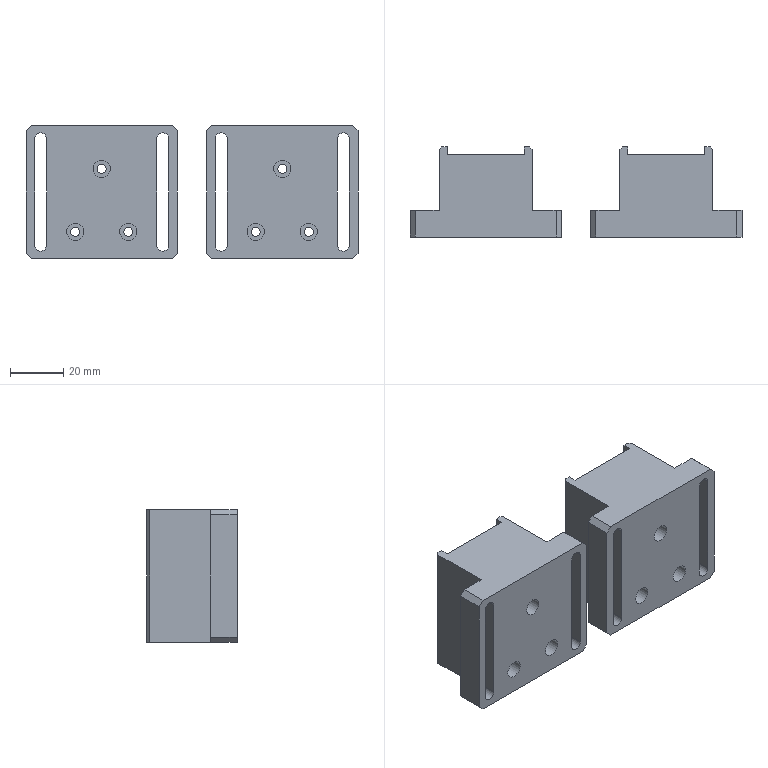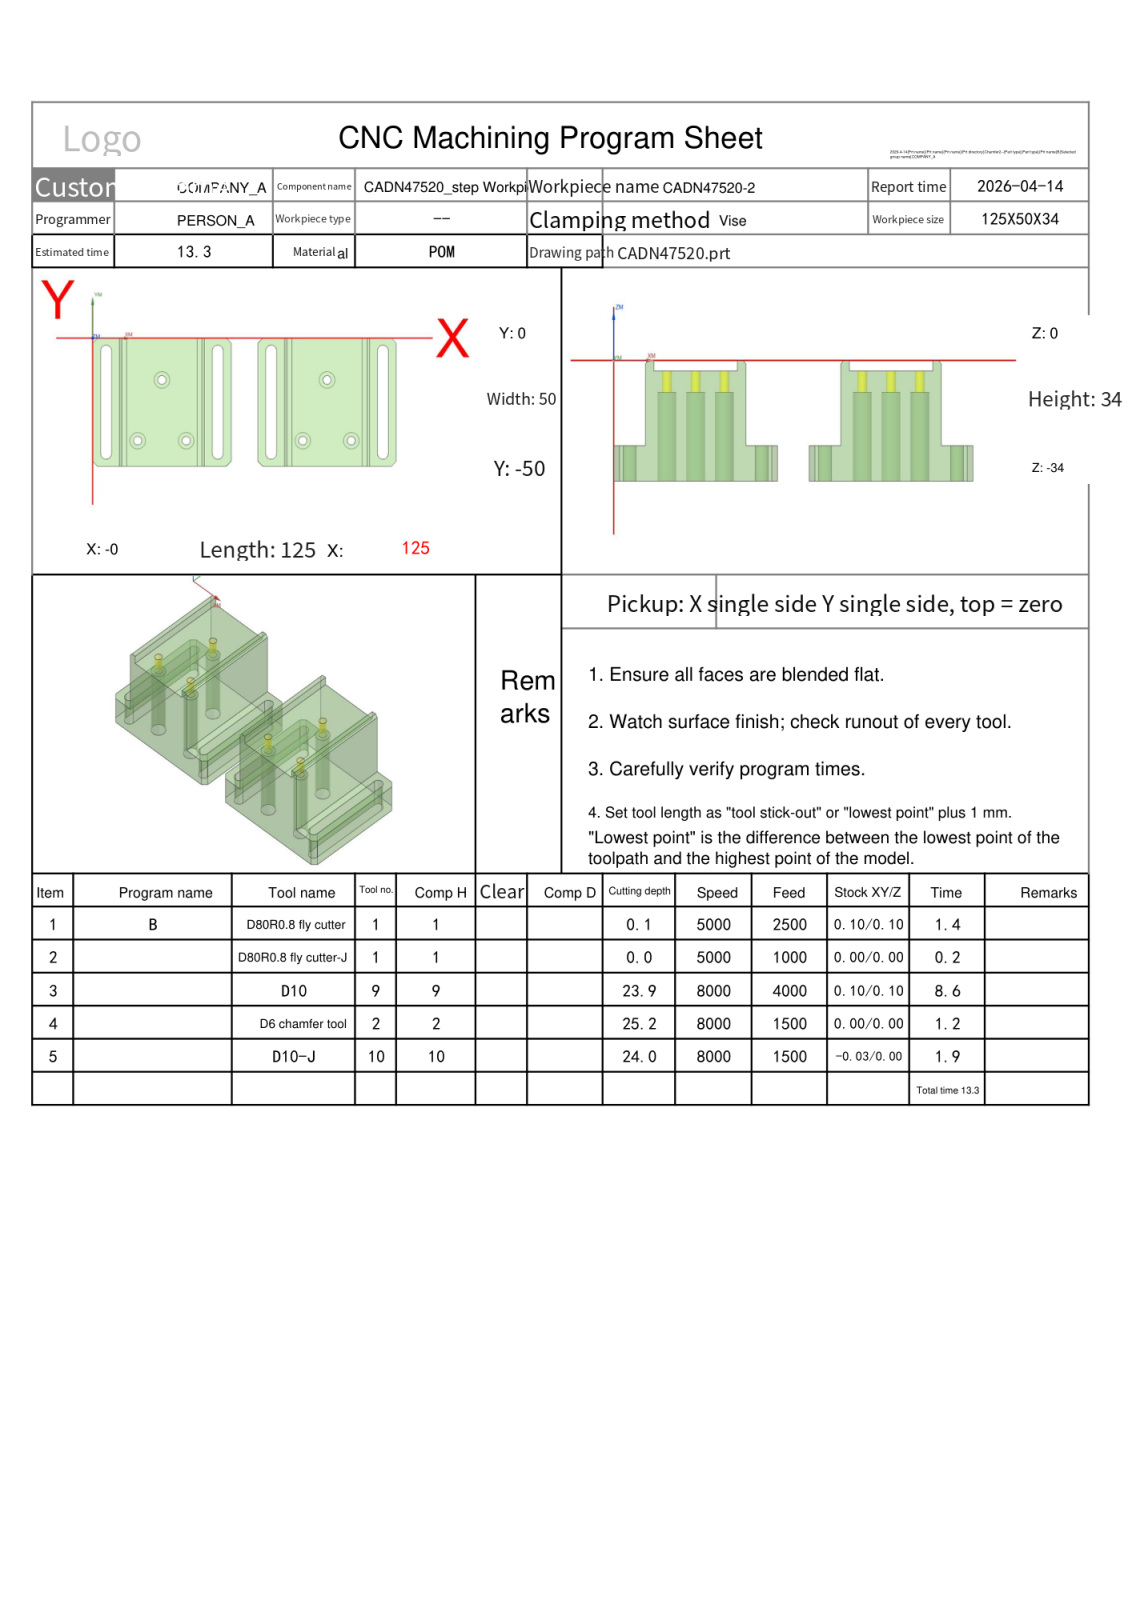NC program | NX | posted by the shop | part box 125 x 34 x 50 mm
Lines 3588 to 4293 of 4293:
N4 T02 M06
(D6 chamfer tool  D=6. R=0. H=02 ce=0.00 di=0.10)
G00 G90 G54 X96.5 Y-16.3 M03 S8000
G43 H02 Z20.
M08
G98 G81 X96.5 Y-16.3 Z-5. R0.0 F1000.
X106.5 Y-40.
X86.5
X38.5
X18.5
X28.5 Y-16.3
G80
G00 Z20.
G00 G90 X79.208 Y.99 M03 S6500
Z20.
Z.13
G01 Z-1.2 F1500.
G03 X79.548 Y.915 I.601 J1.907
G01 X79.602 Y.905
X79.651 Y.928
X79.741 Y.966
X80. Y1.
X82.
G02 X83. Y0.0 I0.0 J-1.
G01 Y-50.
G02 X82. Y-51. I-1. J0.0
G01 X80.
X79.741 Y-50.966
X79.651 Y-50.928
X79.602 Y-50.905
X79.548 Y-50.915
G03 X79.208 Y-50.99 I.261 J-1.983
G01 Z.13
G00 Z10.
X113.792
Z.13
G01 Z-1.2
G03 X113.452 Y-50.915 I-.601 J-1.907
G01 X113.398 Y-50.905
X113.349 Y-50.928
X113.259 Y-50.966
X113. Y-51.
X111.
G02 X110. Y-50. I0.0 J1.
G01 Y-25.
Y0.0
G02 X111. Y1. I1. J0.0
G01 X113.
X113.259 Y.966
X113.349 Y.928
X113.398 Y.905
X113.452 Y.915
G03 X113.792 Y.99 I-.261 J1.983
G01 Z.13
G00 Z10.
X45.792 Y-50.99
Z.13
G01 Z-1.2
G03 X45.452 Y-50.915 I-.601 J-1.907
G01 X45.398 Y-50.905
X45.349 Y-50.928
X45.259 Y-50.966
X45. Y-51.
X43.
G02 X42. Y-50. I0.0 J1.
G01 Y0.0
G02 X43. Y1. I1. J0.0
G01 X45.
X45.259 Y.966
X45.349 Y.928
X45.398 Y.905
X45.452 Y.915
G03 X45.792 Y.99 I-.261 J1.983
G01 Z.13
G00 Z10.
X11.208
Z.13
G01 Z-1.2
G03 X11.548 Y.915 I.601 J1.907
G01 X11.602 Y.905
X11.651 Y.928
X11.741 Y.966
X12. Y1.
X14.
G02 X15. Y0.0 I0.0 J-1.
G01 Y-25.
Y-50.
G02 X14. Y-51. I-1. J0.0
G01 X12.
X11.741 Y-50.966
X11.651 Y-50.928
X11.602 Y-50.905
X11.548 Y-50.915
G03 X11.208 Y-50.99 I.261 J-1.983
G01 Z.13
G00 Z10.
X17.038 Y1.045
Z-1.814
G01 Z-4.2
X17.095 Y1.005
X17.115 Y1.
X39.885
X39.905 Y1.005
X39.962 Y1.045
Z-1.814
G00 Z10.
Y-51.045
Z-1.814
G01 Z-4.2
X39.905 Y-51.005
X39.885 Y-51.
X17.115
X17.095 Y-51.005
X17.038 Y-51.045
Z-1.814
G00 Z10.
X38.912 Y-39.474
Z-2.127
G01 Z-4.2
G03 X38.603 Y-39.314 I-1.075 J-1.687
G01 X38.554 Y-39.29
X38.5 Y-39.3
G03 X37.8 Y-40. I0.0 J-.7
X38.5 Y-40.7 I.7 J0.0
X39.2 Y-40. I0.0 J.7
X38.681 Y-39.324 I-.7 J0.0
G01 X38.5 Y-39.3
X38.446 Y-39.29
X38.397 Y-39.314
G03 X38.088 Y-39.474 I.765 J-1.848
G01 Z-2.624
G00 Z10.
X18.912
Z-2.624
G01 Z-4.2
G03 X18.603 Y-39.314 I-1.075 J-1.687
G01 X18.554 Y-39.29
X18.5 Y-39.3
G03 X17.8 Y-40. I0.0 J-.7
X18.5 Y-40.7 I.7 J0.0
X19.2 Y-40. I0.0 J.7
X18.681 Y-39.324 I-.7 J0.0
G01 X18.5 Y-39.3
X18.446 Y-39.29
X18.397 Y-39.314
G03 X18.088 Y-39.474 I.765 J-1.848
G01 Z-2.127
G00 Z10.
X28.912 Y-15.774
Z-2.624
G01 Z-4.2
G03 X28.603 Y-15.614 I-1.075 J-1.687
G01 X28.554 Y-15.59
X28.5 Y-15.6
G03 X27.8 Y-16.3 I0.0 J-.7
X28.5 Y-17. I.7 J0.0
X29.2 Y-16.3 I0.0 J.7
X28.681 Y-15.624 I-.7 J0.0
G01 X28.5 Y-15.6
X28.446 Y-15.59
X28.397 Y-15.614
G03 X28.088 Y-15.774 I.765 J-1.848
G01 Z-2.624
G00 Z10.
X107.962 Y-51.045
Z-1.814
G01 Z-4.2
X107.905 Y-51.005
X107.885 Y-51.
X85.115
X85.095 Y-51.005
X85.038 Y-51.045
Z-1.814
G00 Z10.
Y1.045
Z-1.814
G01 Z-4.2
X85.095 Y1.005
X85.115 Y1.
X107.885
X107.905 Y1.005
X107.962 Y1.045
Z-1.814
G00 Z10.
X106.912 Y-39.474
Z-2.127
G01 Z-4.2
G03 X106.603 Y-39.314 I-1.075 J-1.687
G01 X106.554 Y-39.29
X106.5 Y-39.3
G03 X105.8 Y-40. I0.0 J-.7
X106.5 Y-40.7 I.7 J0.0
X107.2 Y-40. I0.0 J.7
X106.681 Y-39.324 I-.7 J0.0
G01 X106.5 Y-39.3
X106.446 Y-39.29
X106.397 Y-39.314
G03 X106.088 Y-39.474 I.765 J-1.848
G01 Z-2.624
G00 Z10.
X86.912
Z-2.624
G01 Z-4.2
G03 X86.603 Y-39.314 I-1.075 J-1.687
G01 X86.554 Y-39.29
X86.5 Y-39.3
G03 X85.8 Y-40. I0.0 J-.7
X86.5 Y-40.7 I.7 J0.0
X87.2 Y-40. I0.0 J.7
X86.681 Y-39.324 I-.7 J0.0
G01 X86.5 Y-39.3
X86.446 Y-39.29
X86.397 Y-39.314
G03 X86.088 Y-39.474 I.765 J-1.848
G01 Z-2.127
G00 Z10.
X96.912 Y-15.774
Z-2.624
G01 Z-4.2
G03 X96.603 Y-15.614 I-1.075 J-1.687
G01 X96.554 Y-15.59
X96.5 Y-15.6
G03 X95.8 Y-16.3 I0.0 J-.7
X96.5 Y-17. I.7 J0.0
X97.2 Y-16.3 I0.0 J.7
X96.681 Y-15.624 I-.7 J0.0
G01 X96.5 Y-15.6
X96.446 Y-15.59
X96.397 Y-15.614
G03 X96.088 Y-15.774 I.765 J-1.848
G01 Z-2.624
G00 Z10.
X117.013 Y1.068
Z-2.127
G01 Z-25.2
X117.099 Y1.008
X117.129 Y1.
X123.
X123.259 Y.966
X123.5 Y.866
X123.707 Y.707
X125.707 Y-1.293
X125.866 Y-1.5
X125.966 Y-1.741
X126. Y-2.
Y-48.
X125.966 Y-48.259
X125.866 Y-48.5
X125.707 Y-48.707
X123.707 Y-50.707
X123.5 Y-50.866
X123.259 Y-50.966
X123. Y-51.
X117.129
X117.099 Y-51.008
X117.013 Y-51.068
Z-2.127
G00 Z10.
X118.477 Y-24.614
Z-23.828
G01 Z-25.2
G03 X118.277 Y-24.9 I1.532 J-1.286
G01 X118.247 Y-24.946
X118.25 Y-25.
Y-45.
G03 X119.5 Y-46.25 I1.25 J0.0
X120.75 Y-45. I0.0 J1.25
G01 Y-5.
G03 X119.5 Y-3.75 I-1.25 J0.0
X118.25 Y-5. I0.0 J-1.25
G01 Y-25.
X118.247 Y-25.054
X118.277 Y-25.1
G03 X118.477 Y-25.386 I1.732 J1.
G01 Z-23.828
G00 Z10.
X75.987 Y-51.068
Z-2.127
G01 Z-25.2
X75.901 Y-51.008
X75.871 Y-51.
X70.
X69.741 Y-50.966
X69.5 Y-50.866
X69.293 Y-50.707
X67.293 Y-48.707
X67.134 Y-48.5
X67.034 Y-48.259
X67. Y-48.
Y-2.
X67.034 Y-1.741
X67.134 Y-1.5
X67.293 Y-1.293
X69.293 Y.707
X69.5 Y.866
X69.741 Y.966
X70. Y1.
X75.871
X75.901 Y1.008
X75.987 Y1.068
Z-2.127
G00 Z10.
X72.477 Y-24.614
Z-23.828
G01 Z-25.2
G03 X72.277 Y-24.9 I1.532 J-1.286
G01 X72.247 Y-24.946
X72.25 Y-25.
Y-45.
G03 X73.5 Y-46.25 I1.25 J0.0
X74.75 Y-45. I0.0 J1.25
G01 Y-5.
G03 X73.5 Y-3.75 I-1.25 J0.0
X72.25 Y-5. I0.0 J-1.25
G01 Y-25.
X72.247 Y-25.054
X72.277 Y-25.1
G03 X72.477 Y-25.386 I1.732 J1.
G01 Z-23.828
G00 Z10.
X49.013 Y1.068
Z-2.127
G01 Z-25.2
X49.099 Y1.008
X49.129 Y1.
X55.
X55.259 Y.966
X55.5 Y.866
X55.707 Y.707
X57.707 Y-1.293
X57.866 Y-1.5
X57.966 Y-1.741
X58. Y-2.
Y-48.
X57.966 Y-48.259
X57.866 Y-48.5
X57.707 Y-48.707
X55.707 Y-50.707
X55.5 Y-50.866
X55.259 Y-50.966
X55. Y-51.
X49.129
X49.099 Y-51.008
X49.013 Y-51.068
Z-2.127
G00 Z10.
X50.477 Y-24.614
Z-23.828
G01 Z-25.2
G03 X50.277 Y-24.9 I1.532 J-1.286
G01 X50.247 Y-24.946
X50.25 Y-25.
Y-45.
G03 X51.5 Y-46.25 I1.25 J0.0
X52.75 Y-45. I0.0 J1.25
G01 Y-5.
G03 X51.5 Y-3.75 I-1.25 J0.0
X50.25 Y-5. I0.0 J-1.25
G01 Y-25.
X50.247 Y-25.054
X50.277 Y-25.1
G03 X50.477 Y-25.386 I1.732 J1.
G01 Z-23.828
G00 Z10.
X7.987 Y-51.068
Z-2.127
G01 Z-25.2
X7.901 Y-51.008
X7.871 Y-51.
X2.
X1.741 Y-50.966
X1.5 Y-50.866
X1.293 Y-50.707
X-.707 Y-48.707
X-.866 Y-48.5
X-.966 Y-48.259
X-1. Y-48.
Y-2.
X-.966 Y-1.741
X-.866 Y-1.5
X-.707 Y-1.293
X1.293 Y.707
X1.5 Y.866
X1.741 Y.966
X2. Y1.
X7.871
X7.901 Y1.008
X7.987 Y1.068
Z-2.127
G00 Z10.
X6.523 Y-25.386
Z-23.828
G01 Z-25.2
G03 X6.723 Y-25.1 I-1.532 J1.286
G01 X6.753 Y-25.054
X6.75 Y-25.
Y-5.
G03 X5.5 Y-3.75 I-1.25 J0.0
X4.25 Y-5. I0.0 J-1.25
G01 Y-45.
G03 X5.5 Y-46.25 I1.25 J0.0
X6.75 Y-45. I0.0 J1.25
G01 Y-25.
X6.753 Y-24.946
X6.723 Y-24.9
G03 X6.523 Y-24.614 I-1.732 J-1.
G01 Z-23.828
G00 Z20.
G00 G90 X10.292 Y-52.9 M03 S6500
Z20.
Z-.2
G01 Z-1.7 F1500.
X10.301 Y-52.832
X10.3 Y-52.763
Y2.763
X10.301 Y2.832
X10.292 Y2.9
Z-.2
G00 Z20.
X46.708
Z-.2
G01 Z-1.7
X46.699 Y2.832
X46.7 Y2.763
Y-52.763
X46.699 Y-52.832
X46.708 Y-52.9
Z-.2
G00 Z20.
X78.292
Z-.2
G01 Z-1.7
X78.301 Y-52.832
X78.3 Y-52.763
Y2.763
X78.301 Y2.832
X78.292 Y2.9
Z-.2
G00 Z20.
X114.708
Z-.2
G01 Z-1.7
X114.699 Y2.832
X114.7 Y2.763
Y-52.763
X114.699 Y-52.832
X114.708 Y-52.9
Z-.2
G00 Z20.
G91 G28 Z0.0
M05
M09
G91 G28 Z0.0
M01
N5 T10 M06
(D10-J  D=10. R=0. H=10 ce=0.40 di=0.00)
G00 G90 G54 X127.062 Y5.837 M03 S7000
G43 H10 Z15.8
M08
Z-22.5
G01 Z-24. F1500.
G03 X126. Y4.071 I.938 J-1.766
G01 Y-53.657
G02 X125.707 Y-54.364 I-1. J.001
G01 X125.364 Y-54.707
G02 X124.657 Y-55. I-.707 J.707
G01 X123.699
G02 X122.7 Y-54.001 I.001 J1.
G01 Y4.1
G03 X121.8 Y5. I-.9 J0.0
G01 X120.4
G03 X119.4 Y4. I0.0 J-1.
G01 Y-55.
G03 X121.4 Y-57. I2. J0.0
G01 Z-22.5
G00 Z15.8
X103.599 Y7.
Z-1.5
G01 Z-3.
Y3.
G03 X105.599 Y5. I0.0 J2.
G01 Y-54.1
G02 X104.699 Y-55. I-.9 J0.0
G01 X102.049
G02 X101.049 Y-54. I0.0 J1.
G01 Y4.1
G03 X100.149 Y5. I-.9 J0.0
G01 X97.5
G03 X96.5 Y4. I0.0 J-1.
G01 Y-54.1
G02 X95.6 Y-55. I-.9 J0.0
G01 X92.95
G02 X91.95 Y-54. I0.0 J1.
G01 Y4.1
G03 X91.05 Y5. I-.9 J0.0
G01 X88.4
G03 X87.4 Y4. I0.0 J-1.
G01 Y-55.
G03 X89.4 Y-57. I2. J0.0
G01 Z-1.5
G00 Z15.8
X71.599 Y7.
Z-22.5
G01 Z-24.
Y3.
G03 X73.599 Y5. I0.0 J2.
G01 Y-54.1
G02 X72.699 Y-55. I-.9 J0.0
G01 X70.159
G02 X69.159 Y-54. I0.0 J1.
G01 Y4.001
G03 X68.16 Y5. I-1. J-.001
G01 X67.995
X67.863 Y4.991
X65.586 Y4.686
G03 X64.719 Y3.695 I.133 J-.991
G01 Y-53.669
G02 X63.819 Y-54.569 I-.9 J0.0
G01 X61.28
G02 X60.28 Y-53.569 I0.0 J1.
G01 Y3.695
G03 X59.413 Y4.686 I-1. J-.001
G01 X57.137 Y4.991
X57.005 Y5.
X56.839
G03 X55.84 Y4.001 I.001 J-1.
G01 Y-54.1
G02 X54.94 Y-55. I-.9 J0.0
G01 X52.4
G02 X51.4 Y-54. I0.0 J1.
G01 Y5.
G02 X53.4 Y7. I2. J0.0
G01 Z-22.5
G00 Z1.
X35.599
Z-1.5
G01 Z-3.
Y3.
G03 X37.599 Y5. I0.0 J2.
G01 Y-54.1
G02 X36.699 Y-55. I-.9 J0.0
G01 X34.049
G02 X33.049 Y-54. I0.0 J1.
G01 Y4.1
G03 X32.149 Y5. I-.9 J0.0
G01 X29.5
G03 X28.5 Y4. I0.0 J-1.
G01 Y-54.1
G02 X27.6 Y-55. I-.9 J0.0
G01 X24.95
G02 X23.95 Y-54. I0.0 J1.
G01 Y4.1
G03 X23.05 Y5. I-.9 J0.0
G01 X20.4
G03 X19.4 Y4. I0.0 J-1.
G01 Y-55.
G03 X21.4 Y-57. I2. J0.0
G01 Z-1.5
G00 Z1.
X-2.062 Y-55.837
Z-22.5
G01 Z-24.
G03 X-1. Y-54.071 I-.938 J1.766
G01 Y3.657
G02 X-.708 Y4.364 I1. J-.001
G01 X-.364 Y4.707
G02 X.343 Y5. I.707 J-.707
G01 X1.301
G02 X2.3 Y4.001 I-.001 J-1.
G01 Y-54.1
G03 X3.2 Y-55. I.9 J0.0
G01 X4.6
G03 X5.6 Y-54. I0.0 J1.
G01 Y5.
G03 X3.6 Y7. I-2. J0.0
G01 Z-22.5
G00 Z15.8
G00 G90 X121.199 Y7. M03 S8000
Z15.8
Z-11.
G01 Z-12. F1000.
G41 D10
X120.999
G03 X119. Y5. I.001 J-2.
G01 Y-55.
G03 X120.999 Y-57. I2. J0.0
G01 G40 X121.199
Z-11.
G00 Y7.
Z-23.
G01 Z-24.
G41 D10
X120.999
G03 X119. Y5. I.001 J-2.
G01 Y-55.
G03 X120.999 Y-57. I2. J0.0
G01 G40 X121.199
Z-23.
G00 Z3.
X71.801
Z-11.
G01 Z-12.
G41 D10
X72.001
G03 X74. Y-55. I-.001 J2.
G01 Y5.
G03 X72. Y7. I-2. J0.0
G01 G40 X71.8
Z-11.
G00 X53.2
G01 Z-12.
G41 D10
X53.
G03 X51. Y5. I0.0 J-2.
G01 Y-55.
G03 X52.999 Y-57. I2. J0.0
G01 G40 X53.199
Z-11.
G00 X71.801
Z-23.
G01 Z-24.
G41 D10
X72.001
G03 X74. Y-55. I-.001 J2.
G01 Y5.
G03 X72. Y7. I-2. J0.0
G01 G40 X71.8
Z-23.
G00 X53.2
G01 Z-24.
G41 D10
X53.
G03 X51. Y5. I0.0 J-2.
G01 Y-55.
G03 X52.999 Y-57. I2. J0.0
G01 G40 X53.199
Z-23.
G00 Z3.
X3.801
Z-11.
G01 Z-12.
G41 D10
X4.001
G03 X6. Y-55. I-.001 J2.
G01 Y5.
G03 X4.001 Y7. I-2. J0.0
G01 G40 X3.801
Z-11.
G00 Y-57.
Z-23.
G01 Z-24.
G41 D10
X4.001
G03 X6. Y-55. I-.001 J2.
G01 Y5.
G03 X4.001 Y7. I-2. J0.0
G01 G40 X3.801
Z-23.
G00 Z15.8
G00 G90 X20.857 Y7.007 M03 S8000
Z15.8
Z-2.
G01 Z-3. F1000.
G41 D10
X20.66 Y6.975
G03 X18.975 Y5. I.315 J-1.975
G01 Y-55.
G03 X20.66 Y-56.975 I2. J0.0
G01 G40 X20.857 Y-57.007
Z-2.
G00 X36.143
G01 Z-3.
G41 D10
X36.34 Y-56.975
G03 X38.025 Y-55. I-.315 J1.975
G01 Y5.
G03 X36.34 Y6.975 I-2. J0.0
G01 G40 X36.143 Y7.007
Z-2.
G00 Z3.
X88.857
Z-2.
G01 Z-3.
G41 D10
X88.66 Y6.975
G03 X86.975 Y5. I.315 J-1.975
G01 Y-55.
G03 X88.66 Y-56.975 I2. J0.0
G01 G40 X88.857 Y-57.007
Z-2.
G00 X104.143
G01 Z-3.
G41 D10
X104.34 Y-56.975
G03 X106.025 Y-55. I-.315 J1.975
G01 Y5.
G03 X104.34 Y6.975 I-2. J0.0
G01 G40 X104.143 Y7.007
Z-2.
G00 Z15.8
M05
M09
G91 G28 Z0.0
G91 G28 Y0.0
M30
%